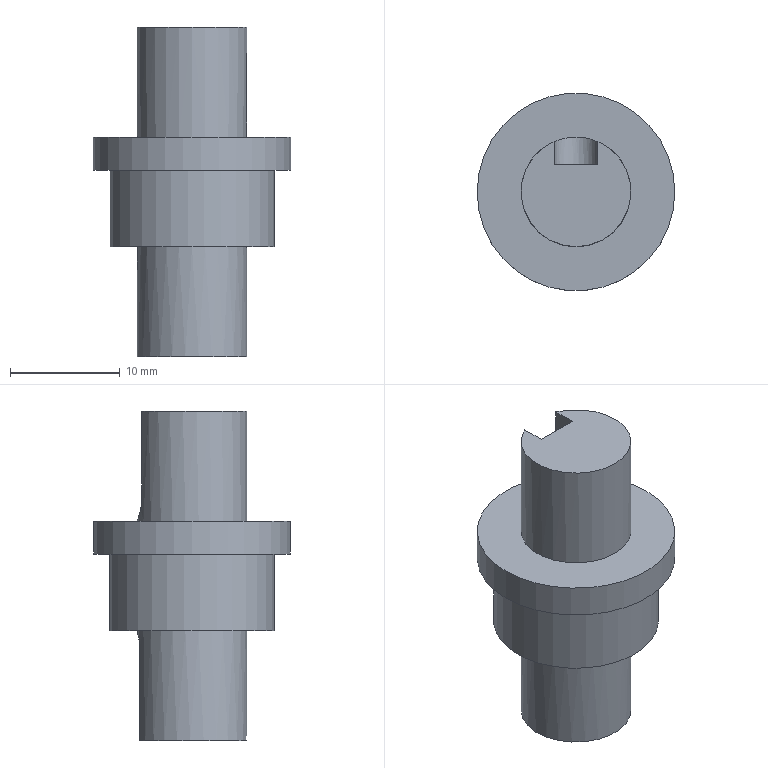Part | NX | features DATUM_CSYS 4, SKETCH 3, EXTRUDE 2, FACE_BLEND 1, HOLE PACKAGE 1, SIMPLE HOLE 1, SUBTRACT 1, SWP104 1, SYMBOLIC_THREAD 1 | 1 solid | 20 faces | box 18 x 18 x 30 mm | volume 3301 mm3 | plane 11 | cylinder 7 | cone 2 | commonest cylinder face diameters 10 x2 3 x1 3.5 x1 4 x1 15 x1 18 x1
STEP:
#1=CARTESIAN_POINT('',(-2.,4.583,30.));
#2=VERTEX_POINT('',#1);
#3=CARTESIAN_POINT('',(-2.,2.5,30.));
#4=VERTEX_POINT('',#3);
#5=CARTESIAN_POINT('',(-2.,12.5,30.));
#6=DIRECTION('',(0.,-1.,0.));
#7=VECTOR('',#6,1000.);
#8=LINE('',#5,#7);
#9=EDGE_CURVE('',#2,#4,#8,.T.);
#10=ORIENTED_EDGE('',*,*,#9,.F.);
#11=CARTESIAN_POINT('',(2.,4.583,30.));
#12=VERTEX_POINT('',#11);
#13=CARTESIAN_POINT('',(0.,0.,30.));
#14=DIRECTION('',(0.,0.,1.));
#15=DIRECTION('',(1.,0.,0.));
#16=AXIS2_PLACEMENT_3D('',#13,#14,#15);
#17=CIRCLE('',#16,5.);
#18=EDGE_CURVE('',#2,#12,#17,.T.);
#19=ORIENTED_EDGE('',*,*,#18,.T.);
#20=CARTESIAN_POINT('',(2.,2.5,30.));
#21=VERTEX_POINT('',#20);
#22=CARTESIAN_POINT('',(2.,2.5,30.));
#23=DIRECTION('',(0.,1.,0.));
#24=VECTOR('',#23,1000.);
#25=LINE('',#22,#24);
#26=EDGE_CURVE('',#21,#12,#25,.T.);
#27=ORIENTED_EDGE('',*,*,#26,.F.);
#28=CARTESIAN_POINT('',(-2.,2.5,30.));
#29=DIRECTION('',(1.,0.,0.));
#30=VECTOR('',#29,1000.);
#31=LINE('',#28,#30);
#32=EDGE_CURVE('',#4,#21,#31,.T.);
#33=ORIENTED_EDGE('',*,*,#32,.F.);
#34=EDGE_LOOP('',(#10,#19,#27,#33));
#35=FACE_BOUND('',#34,.T.);
#36=CARTESIAN_POINT('',(0.,0.,30.));
#37=DIRECTION('',(0.,0.,1.));
#38=DIRECTION('',(1.,0.,0.));
#39=AXIS2_PLACEMENT_3D('',#36,#37,#38);
#40=PLANE('',#39);
#41=ADVANCED_FACE('',(#35),#40,.T.);
#42=CARTESIAN_POINT('',(2.,0.,0.));
#43=VERTEX_POINT('',#42);
#44=CARTESIAN_POINT('',(0.,0.,0.));
#45=DIRECTION('',(0.,0.,1.));
#46=DIRECTION('',(1.,0.,0.));
#47=AXIS2_PLACEMENT_3D('',#44,#45,#46);
#48=CIRCLE('',#47,2.);
#49=EDGE_CURVE('',#43,#43,#48,.T.);
#50=ORIENTED_EDGE('',*,*,#49,.T.);
#51=EDGE_LOOP('',(#50));
#52=FACE_BOUND('',#51,.T.);
#53=CARTESIAN_POINT('',(-1.5,4.77,0.));
#54=VERTEX_POINT('',#53);
#55=CARTESIAN_POINT('',(1.5,4.77,0.));
#56=VERTEX_POINT('',#55);
#57=CARTESIAN_POINT('',(0.,0.,0.));
#58=DIRECTION('',(0.,0.,1.));
#59=DIRECTION('',(1.,0.,0.));
#60=AXIS2_PLACEMENT_3D('',#57,#58,#59);
#61=CIRCLE('',#60,5.);
#62=EDGE_CURVE('',#54,#56,#61,.T.);
#63=ORIENTED_EDGE('',*,*,#62,.F.);
#64=CARTESIAN_POINT('',(-1.5,3.2,0.));
#65=VERTEX_POINT('',#64);
#66=CARTESIAN_POINT('',(-1.5,10.,0.));
#67=DIRECTION('',(0.,-1.,0.));
#68=VECTOR('',#67,1000.);
#69=LINE('',#66,#68);
#70=EDGE_CURVE('',#54,#65,#69,.T.);
#71=ORIENTED_EDGE('',*,*,#70,.T.);
#72=CARTESIAN_POINT('',(1.5,3.2,0.));
#73=VERTEX_POINT('',#72);
#74=CARTESIAN_POINT('',(-1.5,3.2,0.));
#75=DIRECTION('',(1.,0.,0.));
#76=VECTOR('',#75,1000.);
#77=LINE('',#74,#76);
#78=EDGE_CURVE('',#65,#73,#77,.T.);
#79=ORIENTED_EDGE('',*,*,#78,.T.);
#80=CARTESIAN_POINT('',(1.5,10.,0.));
#81=DIRECTION('',(0.,-1.,0.));
#82=VECTOR('',#81,1000.);
#83=LINE('',#80,#82);
#84=EDGE_CURVE('',#56,#73,#83,.T.);
#85=ORIENTED_EDGE('',*,*,#84,.F.);
#86=EDGE_LOOP('',(#63,#71,#79,#85));
#87=FACE_BOUND('',#86,.T.);
#88=CARTESIAN_POINT('',(0.,0.,0.));
#89=DIRECTION('',(0.,0.,1.));
#90=DIRECTION('',(1.,0.,0.));
#91=AXIS2_PLACEMENT_3D('',#88,#89,#90);
#92=PLANE('',#91);
#93=ADVANCED_FACE('',(#52,#87),#92,.F.);
#94=CARTESIAN_POINT('',(-1.5,4.77,8.5));
#95=VERTEX_POINT('',#94);
#96=CARTESIAN_POINT('',(-1.5,4.77,0.));
#97=DIRECTION('',(0.,0.,1.));
#98=VECTOR('',#97,1000.);
#99=LINE('',#96,#98);
#100=EDGE_CURVE('',#54,#95,#99,.T.);
#101=ORIENTED_EDGE('',*,*,#100,.F.);
#102=ORIENTED_EDGE('',*,*,#62,.T.);
#103=CARTESIAN_POINT('',(1.5,4.77,8.5));
#104=VERTEX_POINT('',#103);
#105=CARTESIAN_POINT('',(1.5,4.77,0.));
#106=DIRECTION('',(0.,0.,1.));
#107=VECTOR('',#106,1000.);
#108=LINE('',#105,#107);
#109=EDGE_CURVE('',#104,#56,#108,.F.);
#110=ORIENTED_EDGE('',*,*,#109,.F.);
#111=CARTESIAN_POINT('',(0.,5.,10.));
#112=VERTEX_POINT('',#111);
#113=CARTESIAN_POINT('',(0.,5.,10.));
#114=CARTESIAN_POINT('',(0.7872,5.,10.));
#115=CARTESIAN_POINT('',(1.5,4.77,9.297));
#116=CARTESIAN_POINT('',(1.5,4.77,8.5));
#117=B_SPLINE_CURVE_WITH_KNOTS('',3,(#113,#114,#115,#116),.UNSPECIFIED.,.F.,.F.,(4,4),(0.002359,0.004715),.UNSPECIFIED.);
#118=EDGE_CURVE('',#112,#104,#117,.T.);
#119=ORIENTED_EDGE('',*,*,#118,.F.);
#120=CARTESIAN_POINT('',(0.,0.,10.));
#121=DIRECTION('',(0.,0.,1.));
#122=DIRECTION('',(1.,0.,0.));
#123=AXIS2_PLACEMENT_3D('',#120,#121,#122);
#124=CIRCLE('',#123,5.);
#125=EDGE_CURVE('',#112,#112,#124,.T.);
#126=ORIENTED_EDGE('',*,*,#125,.F.);
#127=CARTESIAN_POINT('',(-1.5,4.77,8.5));
#128=CARTESIAN_POINT('',(-1.5,4.77,9.298));
#129=CARTESIAN_POINT('',(-0.7882,5.,10.));
#130=CARTESIAN_POINT('',(0.,5.,10.));
#131=B_SPLINE_CURVE_WITH_KNOTS('',3,(#127,#128,#129,#130),.UNSPECIFIED.,.F.,.F.,(4,4),(0.,0.002359),.UNSPECIFIED.);
#132=EDGE_CURVE('',#95,#112,#131,.T.);
#133=ORIENTED_EDGE('',*,*,#132,.F.);
#134=EDGE_LOOP('',(#101,#102,#110,#119,#126,#133));
#135=FACE_BOUND('',#134,.T.);
#136=CARTESIAN_POINT('',(0.,0.,0.));
#137=DIRECTION('',(0.,0.,1.));
#138=DIRECTION('',(1.,0.,0.));
#139=AXIS2_PLACEMENT_3D('',#136,#137,#138);
#140=CYLINDRICAL_SURFACE('',#139,5.);
#141=ADVANCED_FACE('',(#135),#140,.T.);
#142=ORIENTED_EDGE('',*,*,#125,.T.);
#143=EDGE_LOOP('',(#142));
#144=FACE_BOUND('',#143,.T.);
#145=CARTESIAN_POINT('',(7.5,0.,10.));
#146=VERTEX_POINT('',#145);
#147=CARTESIAN_POINT('',(0.,0.,10.));
#148=DIRECTION('',(0.,0.,1.));
#149=DIRECTION('',(1.,0.,0.));
#150=AXIS2_PLACEMENT_3D('',#147,#148,#149);
#151=CIRCLE('',#150,7.5);
#152=EDGE_CURVE('',#146,#146,#151,.T.);
#153=ORIENTED_EDGE('',*,*,#152,.F.);
#154=EDGE_LOOP('',(#153));
#155=FACE_BOUND('',#154,.T.);
#156=CARTESIAN_POINT('',(0.,7.5,10.));
#157=DIRECTION('',(0.,0.,-1.));
#158=DIRECTION('',(-1.,0.,0.));
#159=AXIS2_PLACEMENT_3D('',#156,#157,#158);
#160=PLANE('',#159);
#161=ADVANCED_FACE('',(#144,#155),#160,.T.);
#162=ORIENTED_EDGE('',*,*,#152,.T.);
#163=EDGE_LOOP('',(#162));
#164=FACE_BOUND('',#163,.T.);
#165=CARTESIAN_POINT('',(7.5,0.,17.));
#166=VERTEX_POINT('',#165);
#167=CARTESIAN_POINT('',(0.,0.,17.));
#168=DIRECTION('',(0.,0.,1.));
#169=DIRECTION('',(1.,0.,0.));
#170=AXIS2_PLACEMENT_3D('',#167,#168,#169);
#171=CIRCLE('',#170,7.5);
#172=EDGE_CURVE('',#166,#166,#171,.T.);
#173=ORIENTED_EDGE('',*,*,#172,.F.);
#174=EDGE_LOOP('',(#173));
#175=FACE_BOUND('',#174,.T.);
#176=CARTESIAN_POINT('',(0.,0.,0.));
#177=DIRECTION('',(0.,0.,1.));
#178=DIRECTION('',(1.,0.,0.));
#179=AXIS2_PLACEMENT_3D('',#176,#177,#178);
#180=CYLINDRICAL_SURFACE('',#179,7.5);
#181=ADVANCED_FACE('',(#164,#175),#180,.T.);
#182=ORIENTED_EDGE('',*,*,#172,.T.);
#183=EDGE_LOOP('',(#182));
#184=FACE_BOUND('',#183,.T.);
#185=CARTESIAN_POINT('',(9.,0.,17.));
#186=VERTEX_POINT('',#185);
#187=CARTESIAN_POINT('',(0.,0.,17.));
#188=DIRECTION('',(0.,0.,1.));
#189=DIRECTION('',(1.,0.,0.));
#190=AXIS2_PLACEMENT_3D('',#187,#188,#189);
#191=CIRCLE('',#190,9.);
#192=EDGE_CURVE('',#186,#186,#191,.T.);
#193=ORIENTED_EDGE('',*,*,#192,.F.);
#194=EDGE_LOOP('',(#193));
#195=FACE_BOUND('',#194,.T.);
#196=CARTESIAN_POINT('',(0.,9.,17.));
#197=DIRECTION('',(0.,0.,-1.));
#198=DIRECTION('',(-1.,0.,0.));
#199=AXIS2_PLACEMENT_3D('',#196,#197,#198);
#200=PLANE('',#199);
#201=ADVANCED_FACE('',(#184,#195),#200,.T.);
#202=ORIENTED_EDGE('',*,*,#192,.T.);
#203=EDGE_LOOP('',(#202));
#204=FACE_BOUND('',#203,.T.);
#205=CARTESIAN_POINT('',(9.,0.,20.));
#206=VERTEX_POINT('',#205);
#207=CARTESIAN_POINT('',(0.,0.,20.));
#208=DIRECTION('',(0.,0.,1.));
#209=DIRECTION('',(1.,0.,0.));
#210=AXIS2_PLACEMENT_3D('',#207,#208,#209);
#211=CIRCLE('',#210,9.);
#212=EDGE_CURVE('',#206,#206,#211,.T.);
#213=ORIENTED_EDGE('',*,*,#212,.F.);
#214=EDGE_LOOP('',(#213));
#215=FACE_BOUND('',#214,.T.);
#216=CARTESIAN_POINT('',(0.,0.,0.));
#217=DIRECTION('',(0.,0.,1.));
#218=DIRECTION('',(1.,0.,0.));
#219=AXIS2_PLACEMENT_3D('',#216,#217,#218);
#220=CYLINDRICAL_SURFACE('',#219,9.);
#221=ADVANCED_FACE('',(#204,#215),#220,.T.);
#222=CARTESIAN_POINT('',(0.,5.,20.));
#223=VERTEX_POINT('',#222);
#224=CARTESIAN_POINT('',(0.,0.,20.));
#225=DIRECTION('',(0.,0.,1.));
#226=DIRECTION('',(1.,0.,0.));
#227=AXIS2_PLACEMENT_3D('',#224,#225,#226);
#228=CIRCLE('',#227,5.);
#229=EDGE_CURVE('',#223,#223,#228,.T.);
#230=ORIENTED_EDGE('',*,*,#229,.F.);
#231=EDGE_LOOP('',(#230));
#232=FACE_BOUND('',#231,.T.);
#233=ORIENTED_EDGE('',*,*,#212,.T.);
#234=EDGE_LOOP('',(#233));
#235=FACE_BOUND('',#234,.T.);
#236=CARTESIAN_POINT('',(0.,5.,20.));
#237=DIRECTION('',(0.,0.,1.));
#238=DIRECTION('',(1.,0.,0.));
#239=AXIS2_PLACEMENT_3D('',#236,#237,#238);
#240=PLANE('',#239);
#241=ADVANCED_FACE('',(#232,#235),#240,.T.);
#242=CARTESIAN_POINT('',(-2.,4.583,22.));
#243=VERTEX_POINT('',#242);
#244=CARTESIAN_POINT('',(-2.,4.583,0.));
#245=DIRECTION('',(0.,0.,1.));
#246=VECTOR('',#245,1000.);
#247=LINE('',#244,#246);
#248=EDGE_CURVE('',#243,#2,#247,.T.);
#249=ORIENTED_EDGE('',*,*,#248,.F.);
#250=CARTESIAN_POINT('',(0.,5.,20.));
#251=CARTESIAN_POINT('',(-1.056,5.,20.));
#252=CARTESIAN_POINT('',(-2.,4.583,20.932));
#253=CARTESIAN_POINT('',(-2.,4.583,22.));
#254=B_SPLINE_CURVE_WITH_KNOTS('',3,(#250,#251,#252,#253),.UNSPECIFIED.,.F.,.F.,(4,4),(0.003161,0.006317),.UNSPECIFIED.);
#255=EDGE_CURVE('',#223,#243,#254,.T.);
#256=ORIENTED_EDGE('',*,*,#255,.F.);
#257=ORIENTED_EDGE('',*,*,#229,.T.);
#258=CARTESIAN_POINT('',(2.,4.583,22.));
#259=VERTEX_POINT('',#258);
#260=CARTESIAN_POINT('',(2.,4.583,22.));
#261=CARTESIAN_POINT('',(2.,4.583,20.93));
#262=CARTESIAN_POINT('',(1.057,5.,20.));
#263=CARTESIAN_POINT('',(0.,5.,20.));
#264=B_SPLINE_CURVE_WITH_KNOTS('',3,(#260,#261,#262,#263),.UNSPECIFIED.,.F.,.F.,(4,4),(0.,0.003161),.UNSPECIFIED.);
#265=EDGE_CURVE('',#259,#223,#264,.T.);
#266=ORIENTED_EDGE('',*,*,#265,.F.);
#267=CARTESIAN_POINT('',(2.,4.583,0.));
#268=DIRECTION('',(0.,0.,1.));
#269=VECTOR('',#268,1000.);
#270=LINE('',#267,#269);
#271=EDGE_CURVE('',#12,#259,#270,.F.);
#272=ORIENTED_EDGE('',*,*,#271,.F.);
#273=ORIENTED_EDGE('',*,*,#18,.F.);
#274=EDGE_LOOP('',(#249,#256,#257,#266,#272,#273));
#275=FACE_BOUND('',#274,.T.);
#276=CARTESIAN_POINT('',(0.,0.,0.));
#277=DIRECTION('',(0.,0.,1.));
#278=DIRECTION('',(1.,0.,0.));
#279=AXIS2_PLACEMENT_3D('',#276,#277,#278);
#280=CYLINDRICAL_SURFACE('',#279,5.);
#281=ADVANCED_FACE('',(#275),#280,.T.);
#282=CARTESIAN_POINT('',(1.75,0.,13.));
#283=VERTEX_POINT('',#282);
#284=CARTESIAN_POINT('',(0.,0.,13.));
#285=DIRECTION('',(0.,0.,1.));
#286=DIRECTION('',(1.,0.,0.));
#287=AXIS2_PLACEMENT_3D('',#284,#285,#286);
#288=CIRCLE('',#287,1.75);
#289=EDGE_CURVE('',#283,#283,#288,.F.);
#290=ORIENTED_EDGE('',*,*,#289,.T.);
#291=EDGE_LOOP('',(#290));
#292=FACE_BOUND('',#291,.T.);
#293=CARTESIAN_POINT('',(0.,0.,14.052));
#294=VERTEX_POINT('',#293);
#295=VERTEX_LOOP('',#294);
#296=FACE_BOUND('',#295,.T.);
#297=CARTESIAN_POINT('',(0.,0.,13.));
#298=DIRECTION('',(0.,0.,-1.));
#299=DIRECTION('',(-1.,0.,0.));
#300=AXIS2_PLACEMENT_3D('',#297,#298,#299);
#301=CONICAL_SURFACE('',#300,1.75,1.03);
#302=ADVANCED_FACE('',(#292,#296),#301,.F.);
#303=CARTESIAN_POINT('',(1.75,0.,0.25));
#304=VERTEX_POINT('',#303);
#305=CARTESIAN_POINT('',(0.,0.,0.25));
#306=DIRECTION('',(0.,0.,1.));
#307=DIRECTION('',(1.,0.,0.));
#308=AXIS2_PLACEMENT_3D('',#305,#306,#307);
#309=CIRCLE('',#308,1.75);
#310=EDGE_CURVE('',#304,#304,#309,.F.);
#311=ORIENTED_EDGE('',*,*,#310,.T.);
#312=EDGE_LOOP('',(#311));
#313=FACE_BOUND('',#312,.T.);
#314=ORIENTED_EDGE('',*,*,#289,.F.);
#315=EDGE_LOOP('',(#314));
#316=FACE_BOUND('',#315,.T.);
#317=CARTESIAN_POINT('',(0.,0.,0.));
#318=DIRECTION('',(0.,0.,1.));
#319=DIRECTION('',(1.,0.,0.));
#320=AXIS2_PLACEMENT_3D('',#317,#318,#319);
#321=CYLINDRICAL_SURFACE('',#320,1.75);
#322=ADVANCED_FACE('',(#313,#316),#321,.F.);
#323=ORIENTED_EDGE('',*,*,#310,.F.);
#324=EDGE_LOOP('',(#323));
#325=FACE_BOUND('',#324,.T.);
#326=ORIENTED_EDGE('',*,*,#49,.F.);
#327=EDGE_LOOP('',(#326));
#328=FACE_BOUND('',#327,.T.);
#329=CARTESIAN_POINT('',(0.,0.,0.));
#330=DIRECTION('',(0.,0.,-1.));
#331=DIRECTION('',(-1.,0.,0.));
#332=AXIS2_PLACEMENT_3D('',#329,#330,#331);
#333=CONICAL_SURFACE('',#332,2.,0.7854);
#334=ADVANCED_FACE('',(#325,#328),#333,.F.);
#335=ORIENTED_EDGE('',*,*,#100,.T.);
#336=CARTESIAN_POINT('',(-1.5,3.2,8.5));
#337=VERTEX_POINT('',#336);
#338=CARTESIAN_POINT('',(-1.5,10.,8.5));
#339=DIRECTION('',(0.,-1.,0.));
#340=VECTOR('',#339,1000.);
#341=LINE('',#338,#340);
#342=EDGE_CURVE('',#337,#95,#341,.F.);
#343=ORIENTED_EDGE('',*,*,#342,.F.);
#344=CARTESIAN_POINT('',(-1.5,3.2,8.5));
#345=DIRECTION('',(0.,0.,-1.));
#346=VECTOR('',#345,1000.);
#347=LINE('',#344,#346);
#348=EDGE_CURVE('',#65,#337,#347,.F.);
#349=ORIENTED_EDGE('',*,*,#348,.F.);
#350=ORIENTED_EDGE('',*,*,#70,.F.);
#351=EDGE_LOOP('',(#335,#343,#349,#350));
#352=FACE_BOUND('',#351,.T.);
#353=CARTESIAN_POINT('',(-1.5,10.,8.5));
#354=DIRECTION('',(-1.,0.,0.));
#355=DIRECTION('',(0.,0.,1.));
#356=AXIS2_PLACEMENT_3D('',#353,#354,#355);
#357=PLANE('',#356);
#358=ADVANCED_FACE('',(#352),#357,.F.);
#359=ORIENTED_EDGE('',*,*,#109,.T.);
#360=ORIENTED_EDGE('',*,*,#84,.T.);
#361=CARTESIAN_POINT('',(1.5,3.2,8.5));
#362=VERTEX_POINT('',#361);
#363=CARTESIAN_POINT('',(1.5,3.2,0.));
#364=DIRECTION('',(0.,0.,1.));
#365=VECTOR('',#364,1000.);
#366=LINE('',#363,#365);
#367=EDGE_CURVE('',#362,#73,#366,.F.);
#368=ORIENTED_EDGE('',*,*,#367,.F.);
#369=CARTESIAN_POINT('',(1.5,10.,8.5));
#370=DIRECTION('',(0.,-1.,0.));
#371=VECTOR('',#370,1000.);
#372=LINE('',#369,#371);
#373=EDGE_CURVE('',#362,#104,#372,.F.);
#374=ORIENTED_EDGE('',*,*,#373,.T.);
#375=EDGE_LOOP('',(#359,#360,#368,#374));
#376=FACE_BOUND('',#375,.T.);
#377=CARTESIAN_POINT('',(1.5,10.,0.));
#378=DIRECTION('',(1.,0.,0.));
#379=DIRECTION('',(0.,0.,-1.));
#380=AXIS2_PLACEMENT_3D('',#377,#378,#379);
#381=PLANE('',#380);
#382=ADVANCED_FACE('',(#376),#381,.F.);
#383=ORIENTED_EDGE('',*,*,#132,.T.);
#384=ORIENTED_EDGE('',*,*,#118,.T.);
#385=ORIENTED_EDGE('',*,*,#373,.F.);
#386=CARTESIAN_POINT('',(0.,3.2,8.5));
#387=DIRECTION('',(0.,-1.,0.));
#388=DIRECTION('',(1.,0.,0.));
#389=AXIS2_PLACEMENT_3D('',#386,#387,#388);
#390=CIRCLE('',#389,1.5);
#391=EDGE_CURVE('',#337,#362,#390,.F.);
#392=ORIENTED_EDGE('',*,*,#391,.F.);
#393=ORIENTED_EDGE('',*,*,#342,.T.);
#394=EDGE_LOOP('',(#383,#384,#385,#392,#393));
#395=FACE_BOUND('',#394,.T.);
#396=CARTESIAN_POINT('',(0.,10.,8.5));
#397=DIRECTION('',(0.,-1.,0.));
#398=DIRECTION('',(0.,0.,-1.));
#399=AXIS2_PLACEMENT_3D('',#396,#397,#398);
#400=CYLINDRICAL_SURFACE('',#399,1.5);
#401=ADVANCED_FACE('',(#395),#400,.F.);
#402=ORIENTED_EDGE('',*,*,#348,.T.);
#403=ORIENTED_EDGE('',*,*,#391,.T.);
#404=ORIENTED_EDGE('',*,*,#367,.T.);
#405=ORIENTED_EDGE('',*,*,#78,.F.);
#406=EDGE_LOOP('',(#402,#403,#404,#405));
#407=FACE_BOUND('',#406,.T.);
#408=CARTESIAN_POINT('',(0.,3.2,8.5));
#409=DIRECTION('',(0.,-1.,0.));
#410=DIRECTION('',(0.,0.,-1.));
#411=AXIS2_PLACEMENT_3D('',#408,#409,#410);
#412=PLANE('',#411);
#413=ADVANCED_FACE('',(#407),#412,.F.);
#414=ORIENTED_EDGE('',*,*,#265,.T.);
#415=ORIENTED_EDGE('',*,*,#255,.T.);
#416=CARTESIAN_POINT('',(-2.,2.5,22.));
#417=VERTEX_POINT('',#416);
#418=CARTESIAN_POINT('',(-2.,12.5,22.));
#419=DIRECTION('',(0.,1.,0.));
#420=VECTOR('',#419,1000.);
#421=LINE('',#418,#420);
#422=EDGE_CURVE('',#417,#243,#421,.T.);
#423=ORIENTED_EDGE('',*,*,#422,.F.);
#424=CARTESIAN_POINT('',(2.,2.5,22.));
#425=VERTEX_POINT('',#424);
#426=CARTESIAN_POINT('',(0.,2.5,22.));
#427=DIRECTION('',(0.,-1.,0.));
#428=DIRECTION('',(0.,0.,-1.));
#429=AXIS2_PLACEMENT_3D('',#426,#427,#428);
#430=CIRCLE('',#429,2.);
#431=EDGE_CURVE('',#425,#417,#430,.F.);
#432=ORIENTED_EDGE('',*,*,#431,.F.);
#433=CARTESIAN_POINT('',(2.,12.5,22.));
#434=DIRECTION('',(0.,1.,0.));
#435=VECTOR('',#434,1000.);
#436=LINE('',#433,#435);
#437=EDGE_CURVE('',#259,#425,#436,.F.);
#438=ORIENTED_EDGE('',*,*,#437,.F.);
#439=EDGE_LOOP('',(#414,#415,#423,#432,#438));
#440=FACE_BOUND('',#439,.T.);
#441=CARTESIAN_POINT('',(0.,12.5,22.));
#442=DIRECTION('',(0.,-1.,0.));
#443=DIRECTION('',(0.,0.,-1.));
#444=AXIS2_PLACEMENT_3D('',#441,#442,#443);
#445=CYLINDRICAL_SURFACE('',#444,2.);
#446=ADVANCED_FACE('',(#440),#445,.F.);
#447=ORIENTED_EDGE('',*,*,#248,.T.);
#448=ORIENTED_EDGE('',*,*,#9,.T.);
#449=CARTESIAN_POINT('',(-2.,2.5,20.));
#450=DIRECTION('',(0.,0.,1.));
#451=VECTOR('',#450,1000.);
#452=LINE('',#449,#451);
#453=EDGE_CURVE('',#4,#417,#452,.F.);
#454=ORIENTED_EDGE('',*,*,#453,.T.);
#455=ORIENTED_EDGE('',*,*,#422,.T.);
#456=EDGE_LOOP('',(#447,#448,#454,#455));
#457=FACE_BOUND('',#456,.T.);
#458=CARTESIAN_POINT('',(-2.,12.5,20.));
#459=DIRECTION('',(-1.,0.,0.));
#460=DIRECTION('',(0.,-1.,0.));
#461=AXIS2_PLACEMENT_3D('',#458,#459,#460);
#462=PLANE('',#461);
#463=ADVANCED_FACE('',(#457),#462,.F.);
#464=ORIENTED_EDGE('',*,*,#453,.F.);
#465=ORIENTED_EDGE('',*,*,#32,.T.);
#466=CARTESIAN_POINT('',(2.,2.5,20.));
#467=DIRECTION('',(0.,0.,1.));
#468=VECTOR('',#467,1000.);
#469=LINE('',#466,#468);
#470=EDGE_CURVE('',#21,#425,#469,.F.);
#471=ORIENTED_EDGE('',*,*,#470,.T.);
#472=ORIENTED_EDGE('',*,*,#431,.T.);
#473=EDGE_LOOP('',(#464,#465,#471,#472));
#474=FACE_BOUND('',#473,.T.);
#475=CARTESIAN_POINT('',(-2.,2.5,20.));
#476=DIRECTION('',(0.,-1.,0.));
#477=DIRECTION('',(0.,0.,-1.));
#478=AXIS2_PLACEMENT_3D('',#475,#476,#477);
#479=PLANE('',#478);
#480=ADVANCED_FACE('',(#474),#479,.F.);
#481=ORIENTED_EDGE('',*,*,#271,.T.);
#482=ORIENTED_EDGE('',*,*,#437,.T.);
#483=ORIENTED_EDGE('',*,*,#470,.F.);
#484=ORIENTED_EDGE('',*,*,#26,.T.);
#485=EDGE_LOOP('',(#481,#482,#483,#484));
#486=FACE_BOUND('',#485,.T.);
#487=CARTESIAN_POINT('',(2.,2.5,20.));
#488=DIRECTION('',(1.,0.,0.));
#489=DIRECTION('',(0.,1.,0.));
#490=AXIS2_PLACEMENT_3D('',#487,#488,#489);
#491=PLANE('',#490);
#492=ADVANCED_FACE('',(#486),#491,.F.);
#493=CLOSED_SHELL('',(#41,#93,#141,#161,#181,#201,#221,#241,#281,#302,#322,#334,#358,#382,#401,#413,#446,#463,#480,#492));
#494=MANIFOLD_SOLID_BREP('',#493);
#495=(LENGTH_UNIT()NAMED_UNIT(*)SI_UNIT(.MILLI.,.METRE.));
#496=UNCERTAINTY_MEASURE_WITH_UNIT(LENGTH_MEASURE(0.0508),#495,'','');
#497=(NAMED_UNIT(*)PLANE_ANGLE_UNIT()SI_UNIT($,.RADIAN.));
#498=(NAMED_UNIT(*)SI_UNIT($,.STERADIAN.)SOLID_ANGLE_UNIT());
#499=(GEOMETRIC_REPRESENTATION_CONTEXT(3)GLOBAL_UNCERTAINTY_ASSIGNED_CONTEXT((#496))GLOBAL_UNIT_ASSIGNED_CONTEXT((#495,#497,#498))REPRESENTATION_CONTEXT('',''));
#500=ADVANCED_BREP_SHAPE_REPRESENTATION('',(#494),#499);